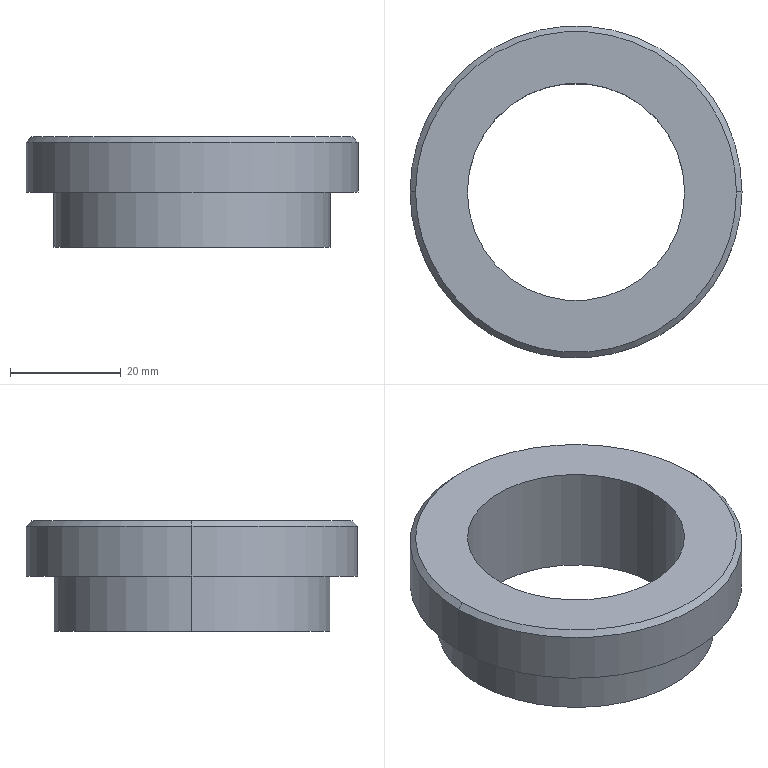Part | SolidWorks | features Chamfer 1, HoleWzd 1, Revolution 1 | 1 solid | 11 faces | box 60 x 60 x 20 mm | volume 23617 mm3 | cylinder 6 | plane 3 | cone 2 | commonest cylinder face diameters 39.25 x2 50 x2 60 x2
STEP:
#1=CARTESIAN_POINT('',(29.,0.,20.));
#2=VERTEX_POINT('',#1);
#3=CARTESIAN_POINT('',(-29.,0.,20.));
#4=VERTEX_POINT('',#3);
#5=CARTESIAN_POINT('',(0.,0.,20.));
#6=DIRECTION('',(0.,0.,1.));
#7=DIRECTION('',(-1.,0.,0.));
#8=AXIS2_PLACEMENT_3D('',#5,#6,#7);
#9=CIRCLE('',#8,29.);
#10=EDGE_CURVE('',#2,#4,#9,.T.);
#11=ORIENTED_EDGE('',*,*,#10,.F.);
#12=CARTESIAN_POINT('',(30.,0.,19.));
#13=VERTEX_POINT('',#12);
#14=CARTESIAN_POINT('',(29.,0.,20.));
#15=DIRECTION('',(0.7071,0.,-0.7071));
#16=VECTOR('',#15,1000.);
#17=LINE('',#14,#16);
#18=EDGE_CURVE('',#2,#13,#17,.T.);
#19=ORIENTED_EDGE('',*,*,#18,.T.);
#20=CARTESIAN_POINT('',(-30.,0.,19.));
#21=VERTEX_POINT('',#20);
#22=CARTESIAN_POINT('',(0.,0.,19.));
#23=DIRECTION('',(0.,0.,-1.));
#24=DIRECTION('',(-1.,0.,0.));
#25=AXIS2_PLACEMENT_3D('',#22,#23,#24);
#26=CIRCLE('',#25,30.);
#27=EDGE_CURVE('',#21,#13,#26,.T.);
#28=ORIENTED_EDGE('',*,*,#27,.F.);
#29=CARTESIAN_POINT('',(-29.,0.,20.));
#30=DIRECTION('',(-0.7071,0.,-0.7071));
#31=VECTOR('',#30,1000.);
#32=LINE('',#29,#31);
#33=EDGE_CURVE('',#4,#21,#32,.T.);
#34=ORIENTED_EDGE('',*,*,#33,.F.);
#35=EDGE_LOOP('',(#11,#19,#28,#34));
#36=FACE_OUTER_BOUND('',#35,.T.);
#37=CARTESIAN_POINT('',(0.,0.,20.));
#38=DIRECTION('',(0.,0.,-1.));
#39=DIRECTION('',(-1.,0.,0.));
#40=AXIS2_PLACEMENT_3D('',#37,#38,#39);
#41=CONICAL_SURFACE('',#40,29.,0.7854);
#42=ADVANCED_FACE('',(#36),#41,.T.);
#43=CARTESIAN_POINT('',(-19.625,0.,0.));
#44=VERTEX_POINT('',#43);
#45=CARTESIAN_POINT('',(19.625,0.,0.));
#46=VERTEX_POINT('',#45);
#47=CARTESIAN_POINT('',(0.,0.,0.));
#48=DIRECTION('',(0.,0.,1.));
#49=DIRECTION('',(1.,0.,0.));
#50=AXIS2_PLACEMENT_3D('',#47,#48,#49);
#51=CIRCLE('',#50,19.625);
#52=EDGE_CURVE('',#44,#46,#51,.T.);
#53=ORIENTED_EDGE('',*,*,#52,.F.);
#54=CARTESIAN_POINT('',(-19.625,0.,20.));
#55=VERTEX_POINT('',#54);
#56=CARTESIAN_POINT('',(-19.625,0.,20.));
#57=DIRECTION('',(0.,0.,1.));
#58=VECTOR('',#57,1000.);
#59=LINE('',#56,#58);
#60=EDGE_CURVE('',#44,#55,#59,.T.);
#61=ORIENTED_EDGE('',*,*,#60,.T.);
#62=CARTESIAN_POINT('',(19.625,0.,20.));
#63=VERTEX_POINT('',#62);
#64=CARTESIAN_POINT('',(0.,0.,20.));
#65=DIRECTION('',(0.,0.,1.));
#66=DIRECTION('',(1.,0.,0.));
#67=AXIS2_PLACEMENT_3D('',#64,#65,#66);
#68=CIRCLE('',#67,19.625);
#69=EDGE_CURVE('',#55,#63,#68,.T.);
#70=ORIENTED_EDGE('',*,*,#69,.T.);
#71=CARTESIAN_POINT('',(19.625,0.,20.));
#72=DIRECTION('',(0.,0.,1.));
#73=VECTOR('',#72,1000.);
#74=LINE('',#71,#73);
#75=EDGE_CURVE('',#46,#63,#74,.T.);
#76=ORIENTED_EDGE('',*,*,#75,.F.);
#77=EDGE_LOOP('',(#53,#61,#70,#76));
#78=FACE_OUTER_BOUND('',#77,.T.);
#79=CARTESIAN_POINT('',(0.,0.,20.));
#80=DIRECTION('',(0.,0.,1.));
#81=DIRECTION('',(1.,0.,0.));
#82=AXIS2_PLACEMENT_3D('',#79,#80,#81);
#83=CYLINDRICAL_SURFACE('',#82,19.625);
#84=ADVANCED_FACE('',(#78),#83,.F.);
#85=CARTESIAN_POINT('',(30.,0.,10.));
#86=VERTEX_POINT('',#85);
#87=CARTESIAN_POINT('',(-30.,0.,10.));
#88=VERTEX_POINT('',#87);
#89=CARTESIAN_POINT('',(0.,0.,10.));
#90=DIRECTION('',(0.,0.,1.));
#91=DIRECTION('',(1.,0.,0.));
#92=AXIS2_PLACEMENT_3D('',#89,#90,#91);
#93=CIRCLE('',#92,30.);
#94=EDGE_CURVE('',#86,#88,#93,.T.);
#95=ORIENTED_EDGE('',*,*,#94,.T.);
#96=CARTESIAN_POINT('',(-30.,0.,20.));
#97=DIRECTION('',(0.,0.,1.));
#98=VECTOR('',#97,1000.);
#99=LINE('',#96,#98);
#100=EDGE_CURVE('',#88,#21,#99,.T.);
#101=ORIENTED_EDGE('',*,*,#100,.T.);
#102=ORIENTED_EDGE('',*,*,#27,.T.);
#103=CARTESIAN_POINT('',(30.,0.,20.));
#104=DIRECTION('',(0.,0.,1.));
#105=VECTOR('',#104,1000.);
#106=LINE('',#103,#105);
#107=EDGE_CURVE('',#86,#13,#106,.T.);
#108=ORIENTED_EDGE('',*,*,#107,.F.);
#109=EDGE_LOOP('',(#95,#101,#102,#108));
#110=FACE_OUTER_BOUND('',#109,.T.);
#111=CARTESIAN_POINT('',(0.,0.,20.));
#112=DIRECTION('',(0.,0.,1.));
#113=DIRECTION('',(1.,0.,0.));
#114=AXIS2_PLACEMENT_3D('',#111,#112,#113);
#115=CYLINDRICAL_SURFACE('',#114,30.);
#116=ADVANCED_FACE('',(#110),#115,.T.);
#117=CARTESIAN_POINT('',(25.,0.,0.));
#118=VERTEX_POINT('',#117);
#119=CARTESIAN_POINT('',(-25.,0.,0.));
#120=VERTEX_POINT('',#119);
#121=CARTESIAN_POINT('',(0.,0.,0.));
#122=DIRECTION('',(0.,0.,1.));
#123=DIRECTION('',(1.,0.,0.));
#124=AXIS2_PLACEMENT_3D('',#121,#122,#123);
#125=CIRCLE('',#124,25.);
#126=EDGE_CURVE('',#118,#120,#125,.T.);
#127=ORIENTED_EDGE('',*,*,#126,.T.);
#128=CARTESIAN_POINT('',(-25.,0.,10.));
#129=VERTEX_POINT('',#128);
#130=CARTESIAN_POINT('',(-25.,0.,20.));
#131=DIRECTION('',(0.,0.,1.));
#132=VECTOR('',#131,1000.);
#133=LINE('',#130,#132);
#134=EDGE_CURVE('',#120,#129,#133,.T.);
#135=ORIENTED_EDGE('',*,*,#134,.T.);
#136=CARTESIAN_POINT('',(25.,0.,10.));
#137=VERTEX_POINT('',#136);
#138=CARTESIAN_POINT('',(0.,0.,10.));
#139=DIRECTION('',(0.,0.,1.));
#140=DIRECTION('',(1.,0.,0.));
#141=AXIS2_PLACEMENT_3D('',#138,#139,#140);
#142=CIRCLE('',#141,25.);
#143=EDGE_CURVE('',#137,#129,#142,.T.);
#144=ORIENTED_EDGE('',*,*,#143,.F.);
#145=CARTESIAN_POINT('',(25.,0.,20.));
#146=DIRECTION('',(0.,0.,1.));
#147=VECTOR('',#146,1000.);
#148=LINE('',#145,#147);
#149=EDGE_CURVE('',#118,#137,#148,.T.);
#150=ORIENTED_EDGE('',*,*,#149,.F.);
#151=EDGE_LOOP('',(#127,#135,#144,#150));
#152=FACE_OUTER_BOUND('',#151,.T.);
#153=CARTESIAN_POINT('',(0.,0.,20.));
#154=DIRECTION('',(0.,0.,1.));
#155=DIRECTION('',(1.,0.,0.));
#156=AXIS2_PLACEMENT_3D('',#153,#154,#155);
#157=CYLINDRICAL_SURFACE('',#156,25.);
#158=ADVANCED_FACE('',(#152),#157,.T.);
#159=CARTESIAN_POINT('',(0.,0.,0.));
#160=DIRECTION('',(0.,0.,1.));
#161=DIRECTION('',(1.,0.,0.));
#162=AXIS2_PLACEMENT_3D('',#159,#160,#161);
#163=CIRCLE('',#162,19.625);
#164=EDGE_CURVE('',#46,#44,#163,.T.);
#165=ORIENTED_EDGE('',*,*,#164,.T.);
#166=ORIENTED_EDGE('',*,*,#52,.T.);
#167=EDGE_LOOP('',(#165,#166));
#168=FACE_BOUND('',#167,.T.);
#169=ORIENTED_EDGE('',*,*,#126,.F.);
#170=CARTESIAN_POINT('',(0.,0.,0.));
#171=DIRECTION('',(0.,0.,1.));
#172=DIRECTION('',(1.,0.,0.));
#173=AXIS2_PLACEMENT_3D('',#170,#171,#172);
#174=CIRCLE('',#173,25.);
#175=EDGE_CURVE('',#120,#118,#174,.T.);
#176=ORIENTED_EDGE('',*,*,#175,.F.);
#177=EDGE_LOOP('',(#169,#176));
#178=FACE_OUTER_BOUND('',#177,.T.);
#179=CARTESIAN_POINT('',(0.,0.,0.));
#180=DIRECTION('',(0.,0.,1.));
#181=DIRECTION('',(1.,0.,0.));
#182=AXIS2_PLACEMENT_3D('',#179,#180,#181);
#183=PLANE('',#182);
#184=ADVANCED_FACE('',(#168,#178),#183,.F.);
#185=ORIENTED_EDGE('',*,*,#134,.F.);
#186=ORIENTED_EDGE('',*,*,#175,.T.);
#187=ORIENTED_EDGE('',*,*,#149,.T.);
#188=CARTESIAN_POINT('',(0.,0.,10.));
#189=DIRECTION('',(0.,0.,1.));
#190=DIRECTION('',(1.,0.,0.));
#191=AXIS2_PLACEMENT_3D('',#188,#189,#190);
#192=CIRCLE('',#191,25.);
#193=EDGE_CURVE('',#129,#137,#192,.T.);
#194=ORIENTED_EDGE('',*,*,#193,.F.);
#195=EDGE_LOOP('',(#185,#186,#187,#194));
#196=FACE_OUTER_BOUND('',#195,.T.);
#197=CARTESIAN_POINT('',(0.,0.,20.));
#198=DIRECTION('',(0.,0.,1.));
#199=DIRECTION('',(1.,0.,0.));
#200=AXIS2_PLACEMENT_3D('',#197,#198,#199);
#201=CYLINDRICAL_SURFACE('',#200,25.);
#202=ADVANCED_FACE('',(#196),#201,.T.);
#203=ORIENTED_EDGE('',*,*,#94,.F.);
#204=CARTESIAN_POINT('',(0.,0.,10.));
#205=DIRECTION('',(0.,0.,1.));
#206=DIRECTION('',(1.,0.,0.));
#207=AXIS2_PLACEMENT_3D('',#204,#205,#206);
#208=CIRCLE('',#207,30.);
#209=EDGE_CURVE('',#88,#86,#208,.T.);
#210=ORIENTED_EDGE('',*,*,#209,.F.);
#211=EDGE_LOOP('',(#203,#210));
#212=FACE_OUTER_BOUND('',#211,.T.);
#213=ORIENTED_EDGE('',*,*,#143,.T.);
#214=ORIENTED_EDGE('',*,*,#193,.T.);
#215=EDGE_LOOP('',(#213,#214));
#216=FACE_BOUND('',#215,.T.);
#217=CARTESIAN_POINT('',(0.,25.,10.));
#218=DIRECTION('',(0.,0.,1.));
#219=DIRECTION('',(1.,0.,0.));
#220=AXIS2_PLACEMENT_3D('',#217,#218,#219);
#221=PLANE('',#220);
#222=ADVANCED_FACE('',(#212,#216),#221,.F.);
#223=ORIENTED_EDGE('',*,*,#100,.F.);
#224=ORIENTED_EDGE('',*,*,#209,.T.);
#225=ORIENTED_EDGE('',*,*,#107,.T.);
#226=CARTESIAN_POINT('',(0.,0.,19.));
#227=DIRECTION('',(0.,0.,-1.));
#228=DIRECTION('',(-1.,0.,0.));
#229=AXIS2_PLACEMENT_3D('',#226,#227,#228);
#230=CIRCLE('',#229,30.);
#231=EDGE_CURVE('',#13,#21,#230,.T.);
#232=ORIENTED_EDGE('',*,*,#231,.T.);
#233=EDGE_LOOP('',(#223,#224,#225,#232));
#234=FACE_OUTER_BOUND('',#233,.T.);
#235=CARTESIAN_POINT('',(0.,0.,20.));
#236=DIRECTION('',(0.,0.,1.));
#237=DIRECTION('',(1.,0.,0.));
#238=AXIS2_PLACEMENT_3D('',#235,#236,#237);
#239=CYLINDRICAL_SURFACE('',#238,30.);
#240=ADVANCED_FACE('',(#234),#239,.T.);
#241=CARTESIAN_POINT('',(0.,0.,20.));
#242=DIRECTION('',(0.,0.,1.));
#243=DIRECTION('',(-1.,0.,0.));
#244=AXIS2_PLACEMENT_3D('',#241,#242,#243);
#245=CIRCLE('',#244,29.);
#246=EDGE_CURVE('',#4,#2,#245,.T.);
#247=ORIENTED_EDGE('',*,*,#246,.T.);
#248=ORIENTED_EDGE('',*,*,#10,.T.);
#249=EDGE_LOOP('',(#247,#248));
#250=FACE_OUTER_BOUND('',#249,.T.);
#251=CARTESIAN_POINT('',(0.,0.,20.));
#252=DIRECTION('',(0.,0.,1.));
#253=DIRECTION('',(1.,0.,0.));
#254=AXIS2_PLACEMENT_3D('',#251,#252,#253);
#255=CIRCLE('',#254,19.625);
#256=EDGE_CURVE('',#63,#55,#255,.T.);
#257=ORIENTED_EDGE('',*,*,#256,.F.);
#258=ORIENTED_EDGE('',*,*,#69,.F.);
#259=EDGE_LOOP('',(#257,#258));
#260=FACE_BOUND('',#259,.T.);
#261=CARTESIAN_POINT('',(0.,30.,20.));
#262=DIRECTION('',(0.,0.,-1.));
#263=DIRECTION('',(-1.,0.,0.));
#264=AXIS2_PLACEMENT_3D('',#261,#262,#263);
#265=PLANE('',#264);
#266=ADVANCED_FACE('',(#250,#260),#265,.F.);
#267=ORIENTED_EDGE('',*,*,#60,.F.);
#268=ORIENTED_EDGE('',*,*,#164,.F.);
#269=ORIENTED_EDGE('',*,*,#75,.T.);
#270=ORIENTED_EDGE('',*,*,#256,.T.);
#271=EDGE_LOOP('',(#267,#268,#269,#270));
#272=FACE_OUTER_BOUND('',#271,.T.);
#273=CARTESIAN_POINT('',(0.,0.,20.));
#274=DIRECTION('',(0.,0.,1.));
#275=DIRECTION('',(1.,0.,0.));
#276=AXIS2_PLACEMENT_3D('',#273,#274,#275);
#277=CYLINDRICAL_SURFACE('',#276,19.625);
#278=ADVANCED_FACE('',(#272),#277,.F.);
#279=ORIENTED_EDGE('',*,*,#18,.F.);
#280=ORIENTED_EDGE('',*,*,#246,.F.);
#281=ORIENTED_EDGE('',*,*,#33,.T.);
#282=ORIENTED_EDGE('',*,*,#231,.F.);
#283=EDGE_LOOP('',(#279,#280,#281,#282));
#284=FACE_OUTER_BOUND('',#283,.T.);
#285=CARTESIAN_POINT('',(0.,0.,20.));
#286=DIRECTION('',(0.,0.,-1.));
#287=DIRECTION('',(-1.,0.,0.));
#288=AXIS2_PLACEMENT_3D('',#285,#286,#287);
#289=CONICAL_SURFACE('',#288,29.,0.7854);
#290=ADVANCED_FACE('',(#284),#289,.T.);
#291=CLOSED_SHELL('',(#42,#84,#116,#158,#184,#202,#222,#240,#266,#278,#290));
#292=MANIFOLD_SOLID_BREP('',#291);
#293=CARTESIAN_POINT('',(0.,0.,0.));
#294=DIRECTION('',(0.,0.,1.));
#295=DIRECTION('',(1.,0.,0.));
#296=AXIS2_PLACEMENT_3D('',#293,#294,#295);
#297=(LENGTH_UNIT()NAMED_UNIT(*)SI_UNIT(.MILLI.,.METRE.));
#298=UNCERTAINTY_MEASURE_WITH_UNIT(LENGTH_MEASURE(0.00001),#297,'','');
#299=(NAMED_UNIT(*)PLANE_ANGLE_UNIT()SI_UNIT($,.RADIAN.));
#300=(NAMED_UNIT(*)SI_UNIT($,.STERADIAN.)SOLID_ANGLE_UNIT());
#301=(GEOMETRIC_REPRESENTATION_CONTEXT(3)GLOBAL_UNCERTAINTY_ASSIGNED_CONTEXT((#298))GLOBAL_UNIT_ASSIGNED_CONTEXT((#297,#299,#300))REPRESENTATION_CONTEXT('',''));
#302=ADVANCED_BREP_SHAPE_REPRESENTATION('',(#292,#296),#301);